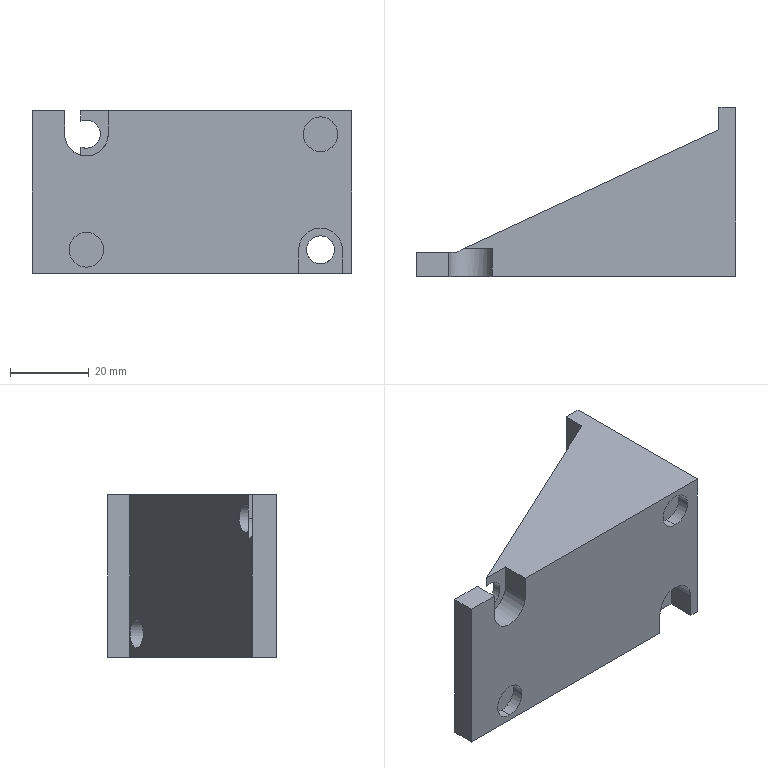Part | STEP file | 4-20.sldasm-Part-218 | 1 solid | 29 faces | box 81.175 x 42.9 x 41.3 mm | volume 66698 mm3 | plane 18 | cylinder 11 | commonest cylinder face diameters 7.142 x5 8.82 x4 11.112 x2
STEP:
#1=CARTESIAN_POINT('',(-270.795,-581.8,-57.11));
#2=VERTEX_POINT('',#1);
#3=CARTESIAN_POINT('',(-270.795,-581.8,-48.29));
#4=VERTEX_POINT('',#3);
#5=CARTESIAN_POINT('',(-270.795,-581.8,-52.7));
#6=DIRECTION('',(0.,1.,0.));
#7=DIRECTION('',(0.,0.,-1.));
#8=AXIS2_PLACEMENT_3D('',#5,#6,#7);
#9=CIRCLE('',#8,4.41);
#10=EDGE_CURVE('',#2,#4,#9,.T.);
#11=ORIENTED_EDGE('',*,*,#10,.F.);
#12=CARTESIAN_POINT('',(-270.795,-578.79,-57.11));
#13=VERTEX_POINT('',#12);
#14=CARTESIAN_POINT('',(-270.795,-583.99,-57.11));
#15=DIRECTION('',(0.,1.,0.));
#16=VECTOR('',#15,1000.);
#17=LINE('',#14,#16);
#18=EDGE_CURVE('',#2,#13,#17,.T.);
#19=ORIENTED_EDGE('',*,*,#18,.T.);
#20=CARTESIAN_POINT('',(-270.795,-578.79,-48.29));
#21=VERTEX_POINT('',#20);
#22=CARTESIAN_POINT('',(-270.795,-578.79,-52.7));
#23=DIRECTION('',(0.,-1.,0.));
#24=DIRECTION('',(0.,0.,-1.));
#25=AXIS2_PLACEMENT_3D('',#22,#23,#24);
#26=CIRCLE('',#25,4.41);
#27=EDGE_CURVE('',#21,#13,#26,.T.);
#28=ORIENTED_EDGE('',*,*,#27,.F.);
#29=CARTESIAN_POINT('',(-270.795,-583.99,-48.29));
#30=DIRECTION('',(0.,1.,0.));
#31=VECTOR('',#30,1000.);
#32=LINE('',#29,#31);
#33=EDGE_CURVE('',#4,#21,#32,.T.);
#34=ORIENTED_EDGE('',*,*,#33,.F.);
#35=EDGE_LOOP('',(#11,#19,#28,#34));
#36=FACE_OUTER_BOUND('',#35,.T.);
#37=CARTESIAN_POINT('',(-270.795,-583.99,-52.7));
#38=DIRECTION('',(0.,1.,0.));
#39=DIRECTION('',(0.,0.,1.));
#40=AXIS2_PLACEMENT_3D('',#37,#38,#39);
#41=CYLINDRICAL_SURFACE('',#40,4.41);
#42=ADVANCED_FACE('',(#36),#41,.F.);
#43=CARTESIAN_POINT('',(-211.295,-581.8,-18.89));
#44=VERTEX_POINT('',#43);
#45=CARTESIAN_POINT('',(-211.295,-581.8,-27.71));
#46=VERTEX_POINT('',#45);
#47=CARTESIAN_POINT('',(-211.295,-581.8,-23.3));
#48=DIRECTION('',(0.,-1.,0.));
#49=DIRECTION('',(0.,0.,-1.));
#50=AXIS2_PLACEMENT_3D('',#47,#48,#49);
#51=CIRCLE('',#50,4.41);
#52=EDGE_CURVE('',#44,#46,#51,.T.);
#53=ORIENTED_EDGE('',*,*,#52,.T.);
#54=CARTESIAN_POINT('',(-211.295,-578.678,-27.71));
#55=VERTEX_POINT('',#54);
#56=CARTESIAN_POINT('',(-211.295,-583.878,-27.71));
#57=DIRECTION('',(0.,1.,0.));
#58=VECTOR('',#57,1000.);
#59=LINE('',#56,#58);
#60=EDGE_CURVE('',#46,#55,#59,.T.);
#61=ORIENTED_EDGE('',*,*,#60,.T.);
#62=CARTESIAN_POINT('',(-211.295,-578.678,-18.89));
#63=VERTEX_POINT('',#62);
#64=CARTESIAN_POINT('',(-211.295,-578.678,-23.3));
#65=DIRECTION('',(0.,1.,0.));
#66=DIRECTION('',(0.,0.,1.));
#67=AXIS2_PLACEMENT_3D('',#64,#65,#66);
#68=CIRCLE('',#67,4.41);
#69=EDGE_CURVE('',#55,#63,#68,.T.);
#70=ORIENTED_EDGE('',*,*,#69,.T.);
#71=CARTESIAN_POINT('',(-211.295,-583.878,-18.89));
#72=DIRECTION('',(0.,1.,0.));
#73=VECTOR('',#72,1000.);
#74=LINE('',#71,#73);
#75=EDGE_CURVE('',#44,#63,#74,.T.);
#76=ORIENTED_EDGE('',*,*,#75,.F.);
#77=EDGE_LOOP('',(#53,#61,#70,#76));
#78=FACE_OUTER_BOUND('',#77,.T.);
#79=CARTESIAN_POINT('',(-211.295,-583.878,-23.3));
#80=DIRECTION('',(0.,1.,0.));
#81=DIRECTION('',(0.,0.,1.));
#82=AXIS2_PLACEMENT_3D('',#79,#80,#81);
#83=CYLINDRICAL_SURFACE('',#82,4.41);
#84=ADVANCED_FACE('',(#78),#83,.F.);
#85=CARTESIAN_POINT('',(-270.795,-574.688,-26.871));
#86=VERTEX_POINT('',#85);
#87=CARTESIAN_POINT('',(-270.795,-574.688,-19.729));
#88=VERTEX_POINT('',#87);
#89=CARTESIAN_POINT('',(-270.795,-574.688,-23.3));
#90=DIRECTION('',(0.,-1.,0.));
#91=DIRECTION('',(0.,0.,-1.));
#92=AXIS2_PLACEMENT_3D('',#89,#90,#91);
#93=CIRCLE('',#92,3.571);
#94=EDGE_CURVE('',#86,#88,#93,.T.);
#95=ORIENTED_EDGE('',*,*,#94,.T.);
#96=CARTESIAN_POINT('',(-270.795,-574.024,-19.729));
#97=VERTEX_POINT('',#96);
#98=CARTESIAN_POINT('',(-270.795,-574.688,-19.729));
#99=DIRECTION('',(0.,1.,0.));
#100=VECTOR('',#99,1000.);
#101=LINE('',#98,#100);
#102=EDGE_CURVE('',#88,#97,#101,.T.);
#103=ORIENTED_EDGE('',*,*,#102,.T.);
#104=CARTESIAN_POINT('',(-270.795,-574.024,-26.871));
#105=VERTEX_POINT('',#104);
#106=CARTESIAN_POINT('',(-270.795,-574.024,-26.871));
#107=CARTESIAN_POINT('',(-263.653,-570.694,-26.871));
#108=CARTESIAN_POINT('',(-263.653,-570.694,-19.729));
#109=CARTESIAN_POINT('',(-270.795,-574.024,-19.729));
#110=(BOUNDED_CURVE()B_SPLINE_CURVE(3,(#106,#107,#108,#109),.UNSPECIFIED.,.F.,.F.)B_SPLINE_CURVE_WITH_KNOTS((4,4),(4.712,7.854),.UNSPECIFIED.)CURVE()GEOMETRIC_REPRESENTATION_ITEM()RATIONAL_B_SPLINE_CURVE((1.,0.3333,0.3333,1.))REPRESENTATION_ITEM(''));
#111=EDGE_CURVE('',#105,#97,#110,.T.);
#112=ORIENTED_EDGE('',*,*,#111,.F.);
#113=CARTESIAN_POINT('',(-270.795,-574.688,-26.871));
#114=DIRECTION('',(0.,1.,0.));
#115=VECTOR('',#114,1000.);
#116=LINE('',#113,#115);
#117=EDGE_CURVE('',#86,#105,#116,.T.);
#118=ORIENTED_EDGE('',*,*,#117,.F.);
#119=EDGE_LOOP('',(#95,#103,#112,#118));
#120=FACE_OUTER_BOUND('',#119,.T.);
#121=CARTESIAN_POINT('',(-270.795,-574.688,-23.3));
#122=DIRECTION('',(0.,1.,0.));
#123=DIRECTION('',(0.,0.,-1.));
#124=AXIS2_PLACEMENT_3D('',#121,#122,#123);
#125=CYLINDRICAL_SURFACE('',#124,3.571);
#126=ADVANCED_FACE('',(#120),#125,.F.);
#127=CARTESIAN_POINT('',(-272.218,-574.688,-26.575));
#128=VERTEX_POINT('',#127);
#129=CARTESIAN_POINT('',(-270.795,-574.688,-23.3));
#130=DIRECTION('',(0.,-1.,0.));
#131=DIRECTION('',(0.,0.,-1.));
#132=AXIS2_PLACEMENT_3D('',#129,#130,#131);
#133=CIRCLE('',#132,3.571);
#134=EDGE_CURVE('',#128,#86,#133,.T.);
#135=ORIENTED_EDGE('',*,*,#134,.T.);
#136=ORIENTED_EDGE('',*,*,#117,.T.);
#137=CARTESIAN_POINT('',(-272.218,-574.688,-26.575));
#138=CARTESIAN_POINT('',(-271.767,-574.478,-26.771));
#139=CARTESIAN_POINT('',(-271.286,-574.254,-26.871));
#140=CARTESIAN_POINT('',(-270.795,-574.024,-26.871));
#141=(BOUNDED_CURVE()B_SPLINE_CURVE(3,(#137,#138,#139,#140),.UNSPECIFIED.,.F.,.T.)B_SPLINE_CURVE_WITH_KNOTS((4,4),(4.303,4.712),.UNSPECIFIED.)CURVE()GEOMETRIC_REPRESENTATION_ITEM()RATIONAL_B_SPLINE_CURVE((1.,0.986,0.986,1.))REPRESENTATION_ITEM(''));
#142=EDGE_CURVE('',#128,#105,#141,.T.);
#143=ORIENTED_EDGE('',*,*,#142,.F.);
#144=EDGE_LOOP('',(#135,#136,#143));
#145=FACE_OUTER_BOUND('',#144,.T.);
#146=CARTESIAN_POINT('',(-270.795,-574.688,-23.3));
#147=DIRECTION('',(0.,1.,0.));
#148=DIRECTION('',(0.,0.,-1.));
#149=AXIS2_PLACEMENT_3D('',#146,#147,#148);
#150=CYLINDRICAL_SURFACE('',#149,3.571);
#151=ADVANCED_FACE('',(#145),#150,.F.);
#152=CARTESIAN_POINT('',(-211.295,-574.688,-56.271));
#153=VERTEX_POINT('',#152);
#154=CARTESIAN_POINT('',(-211.295,-574.688,-49.129));
#155=VERTEX_POINT('',#154);
#156=CARTESIAN_POINT('',(-211.295,-574.688,-52.7));
#157=DIRECTION('',(0.,1.,0.));
#158=DIRECTION('',(0.,0.,1.));
#159=AXIS2_PLACEMENT_3D('',#156,#157,#158);
#160=CIRCLE('',#159,3.571);
#161=EDGE_CURVE('',#153,#155,#160,.T.);
#162=ORIENTED_EDGE('',*,*,#161,.F.);
#163=CARTESIAN_POINT('',(-211.295,-546.279,-56.271));
#164=VERTEX_POINT('',#163);
#165=CARTESIAN_POINT('',(-211.295,-574.688,-56.271));
#166=DIRECTION('',(0.,1.,0.));
#167=VECTOR('',#166,1000.);
#168=LINE('',#165,#167);
#169=EDGE_CURVE('',#153,#164,#168,.T.);
#170=ORIENTED_EDGE('',*,*,#169,.T.);
#171=CARTESIAN_POINT('',(-211.295,-546.279,-49.129));
#172=VERTEX_POINT('',#171);
#173=CARTESIAN_POINT('',(-211.295,-546.279,-49.129));
#174=CARTESIAN_POINT('',(-218.438,-549.61,-49.129));
#175=CARTESIAN_POINT('',(-218.438,-549.61,-56.271));
#176=CARTESIAN_POINT('',(-211.295,-546.279,-56.271));
#177=(BOUNDED_CURVE()B_SPLINE_CURVE(3,(#173,#174,#175,#176),.UNSPECIFIED.,.F.,.F.)B_SPLINE_CURVE_WITH_KNOTS((4,4),(1.571,4.712),.UNSPECIFIED.)CURVE()GEOMETRIC_REPRESENTATION_ITEM()RATIONAL_B_SPLINE_CURVE((1.,0.3333,0.3333,1.))REPRESENTATION_ITEM(''));
#178=EDGE_CURVE('',#172,#164,#177,.T.);
#179=ORIENTED_EDGE('',*,*,#178,.F.);
#180=CARTESIAN_POINT('',(-211.295,-574.688,-49.129));
#181=DIRECTION('',(0.,1.,0.));
#182=VECTOR('',#181,1000.);
#183=LINE('',#180,#182);
#184=EDGE_CURVE('',#155,#172,#183,.T.);
#185=ORIENTED_EDGE('',*,*,#184,.F.);
#186=EDGE_LOOP('',(#162,#170,#179,#185));
#187=FACE_OUTER_BOUND('',#186,.T.);
#188=CARTESIAN_POINT('',(-211.295,-574.688,-52.7));
#189=DIRECTION('',(0.,1.,0.));
#190=DIRECTION('',(0.,0.,1.));
#191=AXIS2_PLACEMENT_3D('',#188,#189,#190);
#192=CYLINDRICAL_SURFACE('',#191,3.571);
#193=ADVANCED_FACE('',(#187),#192,.F.);
#194=ORIENTED_EDGE('',*,*,#52,.F.);
#195=CARTESIAN_POINT('',(-211.295,-581.8,-23.3));
#196=DIRECTION('',(0.,-1.,0.));
#197=DIRECTION('',(0.,0.,-1.));
#198=AXIS2_PLACEMENT_3D('',#195,#196,#197);
#199=CIRCLE('',#198,4.41);
#200=EDGE_CURVE('',#46,#44,#199,.T.);
#201=ORIENTED_EDGE('',*,*,#200,.F.);
#202=EDGE_LOOP('',(#194,#201));
#203=FACE_BOUND('',#202,.T.);
#204=CARTESIAN_POINT('',(-270.795,-581.8,-52.7));
#205=DIRECTION('',(0.,1.,0.));
#206=DIRECTION('',(0.,0.,-1.));
#207=AXIS2_PLACEMENT_3D('',#204,#205,#206);
#208=CIRCLE('',#207,4.41);
#209=EDGE_CURVE('',#4,#2,#208,.T.);
#210=ORIENTED_EDGE('',*,*,#209,.T.);
#211=ORIENTED_EDGE('',*,*,#10,.T.);
#212=EDGE_LOOP('',(#210,#211));
#213=FACE_BOUND('',#212,.T.);
#214=CARTESIAN_POINT('',(-216.851,-581.8,-58.65));
#215=VERTEX_POINT('',#214);
#216=CARTESIAN_POINT('',(-284.545,-581.8,-58.65));
#217=VERTEX_POINT('',#216);
#218=CARTESIAN_POINT('',(-232.845,-581.8,-58.65));
#219=DIRECTION('',(-1.,0.,0.));
#220=VECTOR('',#219,1000.);
#221=LINE('',#218,#220);
#222=EDGE_CURVE('',#215,#217,#221,.T.);
#223=ORIENTED_EDGE('',*,*,#222,.F.);
#224=CARTESIAN_POINT('',(-216.851,-581.8,-52.7));
#225=VERTEX_POINT('',#224);
#226=CARTESIAN_POINT('',(-216.851,-581.8,-64.256));
#227=DIRECTION('',(0.,0.,1.));
#228=VECTOR('',#227,1000.);
#229=LINE('',#226,#228);
#230=EDGE_CURVE('',#215,#225,#229,.T.);
#231=ORIENTED_EDGE('',*,*,#230,.T.);
#232=CARTESIAN_POINT('',(-205.739,-581.8,-52.7));
#233=VERTEX_POINT('',#232);
#234=CARTESIAN_POINT('',(-211.295,-581.8,-52.7));
#235=DIRECTION('',(0.,-1.,0.));
#236=DIRECTION('',(0.,0.,-1.));
#237=AXIS2_PLACEMENT_3D('',#234,#235,#236);
#238=CIRCLE('',#237,5.556);
#239=EDGE_CURVE('',#233,#225,#238,.T.);
#240=ORIENTED_EDGE('',*,*,#239,.F.);
#241=CARTESIAN_POINT('',(-205.739,-581.8,-58.65));
#242=VERTEX_POINT('',#241);
#243=CARTESIAN_POINT('',(-205.739,-581.8,-64.256));
#244=DIRECTION('',(0.,0.,1.));
#245=VECTOR('',#244,1000.);
#246=LINE('',#243,#245);
#247=EDGE_CURVE('',#242,#233,#246,.T.);
#248=ORIENTED_EDGE('',*,*,#247,.F.);
#249=CARTESIAN_POINT('',(-203.37,-581.8,-58.65));
#250=VERTEX_POINT('',#249);
#251=CARTESIAN_POINT('',(-232.845,-581.8,-58.65));
#252=DIRECTION('',(-1.,0.,0.));
#253=VECTOR('',#252,1000.);
#254=LINE('',#251,#253);
#255=EDGE_CURVE('',#250,#242,#254,.T.);
#256=ORIENTED_EDGE('',*,*,#255,.F.);
#257=CARTESIAN_POINT('',(-203.37,-581.8,-17.35));
#258=VERTEX_POINT('',#257);
#259=CARTESIAN_POINT('',(-203.37,-581.8,-38.));
#260=DIRECTION('',(0.,0.,1.));
#261=VECTOR('',#260,1000.);
#262=LINE('',#259,#261);
#263=EDGE_CURVE('',#250,#258,#262,.T.);
#264=ORIENTED_EDGE('',*,*,#263,.T.);
#265=CARTESIAN_POINT('',(-265.239,-581.8,-17.35));
#266=VERTEX_POINT('',#265);
#267=CARTESIAN_POINT('',(-232.845,-581.8,-17.35));
#268=DIRECTION('',(1.,0.,0.));
#269=VECTOR('',#268,1000.);
#270=LINE('',#267,#269);
#271=EDGE_CURVE('',#266,#258,#270,.T.);
#272=ORIENTED_EDGE('',*,*,#271,.F.);
#273=CARTESIAN_POINT('',(-265.239,-581.8,-23.3));
#274=VERTEX_POINT('',#273);
#275=CARTESIAN_POINT('',(-265.239,-581.8,-28.856));
#276=DIRECTION('',(0.,0.,1.));
#277=VECTOR('',#276,1000.);
#278=LINE('',#275,#277);
#279=EDGE_CURVE('',#274,#266,#278,.T.);
#280=ORIENTED_EDGE('',*,*,#279,.F.);
#281=CARTESIAN_POINT('',(-276.351,-581.8,-23.3));
#282=VERTEX_POINT('',#281);
#283=CARTESIAN_POINT('',(-270.795,-581.8,-23.3));
#284=DIRECTION('',(0.,1.,0.));
#285=DIRECTION('',(0.,0.,1.));
#286=AXIS2_PLACEMENT_3D('',#283,#284,#285);
#287=CIRCLE('',#286,5.556);
#288=EDGE_CURVE('',#274,#282,#287,.T.);
#289=ORIENTED_EDGE('',*,*,#288,.T.);
#290=CARTESIAN_POINT('',(-276.351,-581.8,-17.35));
#291=VERTEX_POINT('',#290);
#292=CARTESIAN_POINT('',(-276.351,-581.8,-28.856));
#293=DIRECTION('',(0.,0.,1.));
#294=VECTOR('',#293,1000.);
#295=LINE('',#292,#294);
#296=EDGE_CURVE('',#282,#291,#295,.T.);
#297=ORIENTED_EDGE('',*,*,#296,.T.);
#298=CARTESIAN_POINT('',(-284.545,-581.8,-17.35));
#299=VERTEX_POINT('',#298);
#300=CARTESIAN_POINT('',(-232.845,-581.8,-17.35));
#301=DIRECTION('',(1.,0.,0.));
#302=VECTOR('',#301,1000.);
#303=LINE('',#300,#302);
#304=EDGE_CURVE('',#299,#291,#303,.T.);
#305=ORIENTED_EDGE('',*,*,#304,.F.);
#306=CARTESIAN_POINT('',(-284.545,-581.8,-38.));
#307=DIRECTION('',(0.,0.,1.));
#308=VECTOR('',#307,1000.);
#309=LINE('',#306,#308);
#310=EDGE_CURVE('',#217,#299,#309,.T.);
#311=ORIENTED_EDGE('',*,*,#310,.F.);
#312=EDGE_LOOP('',(#223,#231,#240,#248,#256,#264,#272,#280,#289,#297,#305,#311));
#313=FACE_OUTER_BOUND('',#312,.T.);
#314=CARTESIAN_POINT('',(-232.845,-581.8,-38.));
#315=DIRECTION('',(0.,-1.,0.));
#316=DIRECTION('',(0.,0.,-1.));
#317=AXIS2_PLACEMENT_3D('',#314,#315,#316);
#318=PLANE('',#317);
#319=ADVANCED_FACE('',(#203,#213,#313),#318,.T.);
#320=CARTESIAN_POINT('',(-276.351,-575.7,-17.35));
#321=VERTEX_POINT('',#320);
#322=CARTESIAN_POINT('',(-276.351,-535.,-17.35));
#323=DIRECTION('',(0.,-1.,0.));
#324=VECTOR('',#323,1000.);
#325=LINE('',#322,#324);
#326=EDGE_CURVE('',#321,#291,#325,.T.);
#327=ORIENTED_EDGE('',*,*,#326,.F.);
#328=CARTESIAN_POINT('',(-284.545,-575.7,-17.35));
#329=VERTEX_POINT('',#328);
#330=CARTESIAN_POINT('',(-246.645,-575.7,-17.35));
#331=DIRECTION('',(-1.,0.,0.));
#332=VECTOR('',#331,1000.);
#333=LINE('',#330,#332);
#334=EDGE_CURVE('',#321,#329,#333,.T.);
#335=ORIENTED_EDGE('',*,*,#334,.T.);
#336=CARTESIAN_POINT('',(-284.545,-535.,-17.35));
#337=DIRECTION('',(0.,-1.,0.));
#338=VECTOR('',#337,1000.);
#339=LINE('',#336,#338);
#340=EDGE_CURVE('',#329,#299,#339,.T.);
#341=ORIENTED_EDGE('',*,*,#340,.T.);
#342=ORIENTED_EDGE('',*,*,#304,.T.);
#343=EDGE_LOOP('',(#327,#335,#341,#342));
#344=FACE_OUTER_BOUND('',#343,.T.);
#345=CARTESIAN_POINT('',(-232.845,-535.,-17.35));
#346=DIRECTION('',(0.,0.,1.));
#347=DIRECTION('',(0.,-1.,0.));
#348=AXIS2_PLACEMENT_3D('',#345,#346,#347);
#349=PLANE('',#348);
#350=ADVANCED_FACE('',(#344),#349,.T.);
#351=CARTESIAN_POINT('',(-276.351,-575.7,-23.3));
#352=VERTEX_POINT('',#351);
#353=CARTESIAN_POINT('',(-276.351,-578.244,-23.3));
#354=DIRECTION('',(0.,-1.,0.));
#355=VECTOR('',#354,1000.);
#356=LINE('',#353,#355);
#357=EDGE_CURVE('',#352,#282,#356,.T.);
#358=ORIENTED_EDGE('',*,*,#357,.T.);
#359=ORIENTED_EDGE('',*,*,#288,.F.);
#360=CARTESIAN_POINT('',(-265.239,-574.688,-23.3));
#361=VERTEX_POINT('',#360);
#362=CARTESIAN_POINT('',(-265.239,-578.244,-23.3));
#363=DIRECTION('',(0.,1.,0.));
#364=VECTOR('',#363,1000.);
#365=LINE('',#362,#364);
#366=EDGE_CURVE('',#274,#361,#365,.T.);
#367=ORIENTED_EDGE('',*,*,#366,.T.);
#368=CARTESIAN_POINT('',(-272.218,-574.688,-28.671));
#369=VERTEX_POINT('',#368);
#370=CARTESIAN_POINT('',(-270.795,-574.688,-23.3));
#371=DIRECTION('',(0.,1.,0.));
#372=DIRECTION('',(0.,0.,1.));
#373=AXIS2_PLACEMENT_3D('',#370,#371,#372);
#374=CIRCLE('',#373,5.556);
#375=EDGE_CURVE('',#361,#369,#374,.T.);
#376=ORIENTED_EDGE('',*,*,#375,.T.);
#377=CARTESIAN_POINT('',(-274.388,-575.7,-27.538));
#378=VERTEX_POINT('',#377);
#379=CARTESIAN_POINT('',(-274.388,-575.7,-27.538));
#380=CARTESIAN_POINT('',(-273.756,-575.405,-28.074));
#381=CARTESIAN_POINT('',(-273.02,-575.062,-28.458));
#382=CARTESIAN_POINT('',(-272.218,-574.688,-28.671));
#383=(BOUNDED_CURVE()B_SPLINE_CURVE(3,(#379,#380,#381,#382),.UNSPECIFIED.,.F.,.F.)B_SPLINE_CURVE_WITH_KNOTS((4,4),(0.8675,1.312),.UNSPECIFIED.)CURVE()GEOMETRIC_REPRESENTATION_ITEM()RATIONAL_B_SPLINE_CURVE((1.,0.9836,0.9836,1.))REPRESENTATION_ITEM(''));
#384=EDGE_CURVE('',#378,#369,#383,.T.);
#385=ORIENTED_EDGE('',*,*,#384,.F.);
#386=CARTESIAN_POINT('',(-270.795,-575.7,-23.3));
#387=DIRECTION('',(0.,-1.,0.));
#388=DIRECTION('',(0.,0.,-1.));
#389=AXIS2_PLACEMENT_3D('',#386,#387,#388);
#390=CIRCLE('',#389,5.556);
#391=EDGE_CURVE('',#352,#378,#390,.T.);
#392=ORIENTED_EDGE('',*,*,#391,.F.);
#393=EDGE_LOOP('',(#358,#359,#367,#376,#385,#392));
#394=FACE_OUTER_BOUND('',#393,.T.);
#395=CARTESIAN_POINT('',(-270.795,-574.688,-23.3));
#396=DIRECTION('',(0.,-1.,0.));
#397=DIRECTION('',(0.,0.,1.));
#398=AXIS2_PLACEMENT_3D('',#395,#396,#397);
#399=CYLINDRICAL_SURFACE('',#398,5.556);
#400=ADVANCED_FACE('',(#394),#399,.F.);
#401=CARTESIAN_POINT('',(-216.851,-574.688,-58.65));
#402=VERTEX_POINT('',#401);
#403=CARTESIAN_POINT('',(-216.851,-535.,-58.65));
#404=DIRECTION('',(0.,1.,0.));
#405=VECTOR('',#404,1000.);
#406=LINE('',#403,#405);
#407=EDGE_CURVE('',#215,#402,#406,.T.);
#408=ORIENTED_EDGE('',*,*,#407,.F.);
#409=ORIENTED_EDGE('',*,*,#222,.T.);
#410=CARTESIAN_POINT('',(-284.545,-575.7,-58.65));
#411=VERTEX_POINT('',#410);
#412=CARTESIAN_POINT('',(-284.545,-535.,-58.65));
#413=DIRECTION('',(0.,-1.,0.));
#414=VECTOR('',#413,1000.);
#415=LINE('',#412,#414);
#416=EDGE_CURVE('',#411,#217,#415,.T.);
#417=ORIENTED_EDGE('',*,*,#416,.F.);
#418=CARTESIAN_POINT('',(-274.388,-575.7,-58.65));
#419=VERTEX_POINT('',#418);
#420=CARTESIAN_POINT('',(-246.645,-575.7,-58.65));
#421=DIRECTION('',(1.,0.,0.));
#422=VECTOR('',#421,1000.);
#423=LINE('',#420,#422);
#424=EDGE_CURVE('',#411,#419,#423,.T.);
#425=ORIENTED_EDGE('',*,*,#424,.T.);
#426=CARTESIAN_POINT('',(-207.645,-544.577,-58.65));
#427=VERTEX_POINT('',#426);
#428=CARTESIAN_POINT('',(-243.748,-561.412,-58.65));
#429=DIRECTION('',(-0.9063,-0.4226,0.));
#430=VECTOR('',#429,1000.);
#431=LINE('',#428,#430);
#432=EDGE_CURVE('',#427,#419,#431,.T.);
#433=ORIENTED_EDGE('',*,*,#432,.F.);
#434=CARTESIAN_POINT('',(-207.645,-538.9,-58.65));
#435=VERTEX_POINT('',#434);
#436=CARTESIAN_POINT('',(-207.645,-555.2,-58.65));
#437=DIRECTION('',(0.,1.,0.));
#438=VECTOR('',#437,1000.);
#439=LINE('',#436,#438);
#440=EDGE_CURVE('',#427,#435,#439,.T.);
#441=ORIENTED_EDGE('',*,*,#440,.T.);
#442=CARTESIAN_POINT('',(-203.37,-538.9,-58.65));
#443=VERTEX_POINT('',#442);
#444=CARTESIAN_POINT('',(-232.845,-538.9,-58.65));
#445=DIRECTION('',(1.,0.,0.));
#446=VECTOR('',#445,1000.);
#447=LINE('',#444,#446);
#448=EDGE_CURVE('',#435,#443,#447,.T.);
#449=ORIENTED_EDGE('',*,*,#448,.T.);
#450=CARTESIAN_POINT('',(-203.37,-535.,-58.65));
#451=DIRECTION('',(0.,-1.,0.));
#452=VECTOR('',#451,1000.);
#453=LINE('',#450,#452);
#454=EDGE_CURVE('',#443,#250,#453,.T.);
#455=ORIENTED_EDGE('',*,*,#454,.T.);
#456=ORIENTED_EDGE('',*,*,#255,.T.);
#457=CARTESIAN_POINT('',(-205.739,-574.688,-58.65));
#458=VERTEX_POINT('',#457);
#459=CARTESIAN_POINT('',(-205.739,-535.,-58.65));
#460=DIRECTION('',(0.,-1.,0.));
#461=VECTOR('',#460,1000.);
#462=LINE('',#459,#461);
#463=EDGE_CURVE('',#458,#242,#462,.T.);
#464=ORIENTED_EDGE('',*,*,#463,.F.);
#465=CARTESIAN_POINT('',(-232.845,-574.688,-58.65));
#466=DIRECTION('',(1.,0.,0.));
#467=VECTOR('',#466,1000.);
#468=LINE('',#465,#467);
#469=EDGE_CURVE('',#402,#458,#468,.T.);
#470=ORIENTED_EDGE('',*,*,#469,.F.);
#471=EDGE_LOOP('',(#408,#409,#417,#425,#433,#441,#449,#455,#456,#464,#470));
#472=FACE_OUTER_BOUND('',#471,.T.);
#473=CARTESIAN_POINT('',(-232.845,-535.,-58.65));
#474=DIRECTION('',(0.,0.,-1.));
#475=DIRECTION('',(0.,1.,0.));
#476=AXIS2_PLACEMENT_3D('',#473,#474,#475);
#477=PLANE('',#476);
#478=ADVANCED_FACE('',(#472),#477,.T.);
#479=CARTESIAN_POINT('',(-265.239,-574.688,-17.35));
#480=VERTEX_POINT('',#479);
#481=CARTESIAN_POINT('',(-272.218,-574.688,-17.35));
#482=VERTEX_POINT('',#481);
#483=CARTESIAN_POINT('',(-232.845,-574.688,-17.35));
#484=DIRECTION('',(-1.,0.,0.));
#485=VECTOR('',#484,1000.);
#486=LINE('',#483,#485);
#487=EDGE_CURVE('',#480,#482,#486,.T.);
#488=ORIENTED_EDGE('',*,*,#487,.F.);
#489=CARTESIAN_POINT('',(-265.239,-535.,-17.35));
#490=DIRECTION('',(0.,1.,0.));
#491=VECTOR('',#490,1000.);
#492=LINE('',#489,#491);
#493=EDGE_CURVE('',#266,#480,#492,.T.);
#494=ORIENTED_EDGE('',*,*,#493,.F.);
#495=ORIENTED_EDGE('',*,*,#271,.T.);
#496=CARTESIAN_POINT('',(-203.37,-538.9,-17.35));
#497=VERTEX_POINT('',#496);
#498=CARTESIAN_POINT('',(-203.37,-535.,-17.35));
#499=DIRECTION('',(0.,1.,0.));
#500=VECTOR('',#499,1000.);
#501=LINE('',#498,#500);
#502=EDGE_CURVE('',#258,#497,#501,.T.);
#503=ORIENTED_EDGE('',*,*,#502,.T.);
#504=CARTESIAN_POINT('',(-207.645,-538.9,-17.35));
#505=VERTEX_POINT('',#504);
#506=CARTESIAN_POINT('',(-232.845,-538.9,-17.35));
#507=DIRECTION('',(-1.,0.,0.));
#508=VECTOR('',#507,1000.);
#509=LINE('',#506,#508);
#510=EDGE_CURVE('',#497,#505,#509,.T.);
#511=ORIENTED_EDGE('',*,*,#510,.T.);
#512=CARTESIAN_POINT('',(-207.645,-544.577,-17.35));
#513=VERTEX_POINT('',#512);
#514=CARTESIAN_POINT('',(-207.645,-555.2,-17.35));
#515=DIRECTION('',(0.,-1.,0.));
#516=VECTOR('',#515,1000.);
#517=LINE('',#514,#516);
#518=EDGE_CURVE('',#505,#513,#517,.T.);
#519=ORIENTED_EDGE('',*,*,#518,.T.);
#520=CARTESIAN_POINT('',(-243.748,-561.412,-17.35));
#521=DIRECTION('',(0.9063,0.4226,0.));
#522=VECTOR('',#521,1000.);
#523=LINE('',#520,#522);
#524=EDGE_CURVE('',#482,#513,#523,.T.);
#525=ORIENTED_EDGE('',*,*,#524,.F.);
#526=EDGE_LOOP('',(#488,#494,#495,#503,#511,#519,#525));
#527=FACE_OUTER_BOUND('',#526,.T.);
#528=CARTESIAN_POINT('',(-232.845,-535.,-17.35));
#529=DIRECTION('',(0.,0.,1.));
#530=DIRECTION('',(0.,-1.,0.));
#531=AXIS2_PLACEMENT_3D('',#528,#529,#530);
#532=PLANE('',#531);
#533=ADVANCED_FACE('',(#527),#532,.T.);
#534=CARTESIAN_POINT('',(-207.645,-538.9,-38.));
#535=DIRECTION('',(0.,0.,-1.));
#536=VECTOR('',#535,1000.);
#537=LINE('',#534,#536);
#538=EDGE_CURVE('',#505,#435,#537,.T.);
#539=ORIENTED_EDGE('',*,*,#538,.F.);
#540=ORIENTED_EDGE('',*,*,#510,.F.);
#541=CARTESIAN_POINT('',(-203.37,-538.9,-38.));
#542=DIRECTION('',(0.,0.,-1.));
#543=VECTOR('',#542,1000.);
#544=LINE('',#541,#543);
#545=EDGE_CURVE('',#497,#443,#544,.T.);
#546=ORIENTED_EDGE('',*,*,#545,.T.);
#547=ORIENTED_EDGE('',*,*,#448,.F.);
#548=EDGE_LOOP('',(#539,#540,#546,#547));
#549=FACE_OUTER_BOUND('',#548,.T.);
#550=CARTESIAN_POINT('',(-232.845,-538.9,-38.));
#551=DIRECTION('',(0.,1.,0.));
#552=DIRECTION('',(0.,0.,1.));
#553=AXIS2_PLACEMENT_3D('',#550,#551,#552);
#554=PLANE('',#553);
#555=ADVANCED_FACE('',(#549),#554,.T.);
#556=ORIENTED_EDGE('',*,*,#263,.F.);
#557=ORIENTED_EDGE('',*,*,#454,.F.);
#558=ORIENTED_EDGE('',*,*,#545,.F.);
#559=ORIENTED_EDGE('',*,*,#502,.F.);
#560=EDGE_LOOP('',(#556,#557,#558,#559));
#561=FACE_OUTER_BOUND('',#560,.T.);
#562=CARTESIAN_POINT('',(-203.37,-558.4,-38.));
#563=DIRECTION('',(1.,0.,0.));
#564=DIRECTION('',(0.,-1.,0.));
#565=AXIS2_PLACEMENT_3D('',#562,#563,#564);
#566=PLANE('',#565);
#567=ADVANCED_FACE('',(#561),#566,.T.);
#568=CARTESIAN_POINT('',(-284.545,-575.7,-38.));
#569=DIRECTION('',(0.,0.,1.));
#570=VECTOR('',#569,1000.);
#571=LINE('',#568,#570);
#572=EDGE_CURVE('',#411,#329,#571,.T.);
#573=ORIENTED_EDGE('',*,*,#572,.F.);
#574=ORIENTED_EDGE('',*,*,#416,.T.);
#575=ORIENTED_EDGE('',*,*,#310,.T.);
#576=ORIENTED_EDGE('',*,*,#340,.F.);
#577=EDGE_LOOP('',(#573,#574,#575,#576));
#578=FACE_OUTER_BOUND('',#577,.T.);
#579=CARTESIAN_POINT('',(-284.545,-535.,-38.));
#580=DIRECTION('',(-1.,0.,0.));
#581=DIRECTION('',(0.,1.,0.));
#582=AXIS2_PLACEMENT_3D('',#579,#580,#581);
#583=PLANE('',#582);
#584=ADVANCED_FACE('',(#578),#583,.T.);
#585=ORIENTED_EDGE('',*,*,#334,.F.);
#586=CARTESIAN_POINT('',(-276.351,-575.7,-58.65));
#587=DIRECTION('',(0.,0.,-1.));
#588=VECTOR('',#587,1000.);
#589=LINE('',#586,#588);
#590=EDGE_CURVE('',#321,#352,#589,.T.);
#591=ORIENTED_EDGE('',*,*,#590,.T.);
#592=ORIENTED_EDGE('',*,*,#391,.T.);
#593=CARTESIAN_POINT('',(-274.388,-575.7,-58.65));
#594=DIRECTION('',(0.,0.,1.));
#595=VECTOR('',#594,1000.);
#596=LINE('',#593,#595);
#597=EDGE_CURVE('',#419,#378,#596,.T.);
#598=ORIENTED_EDGE('',*,*,#597,.F.);
#599=ORIENTED_EDGE('',*,*,#424,.F.);
#600=ORIENTED_EDGE('',*,*,#572,.T.);
#601=EDGE_LOOP('',(#585,#591,#592,#598,#599,#600));
#602=FACE_OUTER_BOUND('',#601,.T.);
#603=CARTESIAN_POINT('',(-246.645,-575.7,-58.65));
#604=DIRECTION('',(0.,-1.,0.));
#605=DIRECTION('',(0.,0.,-1.));
#606=AXIS2_PLACEMENT_3D('',#603,#604,#605);
#607=PLANE('',#606);
#608=ADVANCED_FACE('',(#602),#607,.F.);
#609=CARTESIAN_POINT('',(-272.218,-574.688,-20.025));
#610=VERTEX_POINT('',#609);
#611=CARTESIAN_POINT('',(-272.218,-574.688,-58.65));
#612=DIRECTION('',(0.,0.,1.));
#613=VECTOR('',#612,1000.);
#614=LINE('',#611,#613);
#615=EDGE_CURVE('',#610,#482,#614,.T.);
#616=ORIENTED_EDGE('',*,*,#615,.T.);
#617=ORIENTED_EDGE('',*,*,#524,.T.);
#618=CARTESIAN_POINT('',(-207.645,-544.577,-58.65));
#619=DIRECTION('',(0.,0.,-1.));
#620=VECTOR('',#619,1000.);
#621=LINE('',#618,#620);
#622=EDGE_CURVE('',#513,#427,#621,.T.);
#623=ORIENTED_EDGE('',*,*,#622,.T.);
#624=ORIENTED_EDGE('',*,*,#432,.T.);
#625=ORIENTED_EDGE('',*,*,#597,.T.);
#626=ORIENTED_EDGE('',*,*,#384,.T.);
#627=CARTESIAN_POINT('',(-272.218,-574.688,-58.65));
#628=DIRECTION('',(0.,0.,1.));
#629=VECTOR('',#628,1000.);
#630=LINE('',#627,#629);
#631=EDGE_CURVE('',#369,#128,#630,.T.);
#632=ORIENTED_EDGE('',*,*,#631,.T.);
#633=ORIENTED_EDGE('',*,*,#142,.T.);
#634=ORIENTED_EDGE('',*,*,#111,.T.);
#635=CARTESIAN_POINT('',(-270.795,-574.024,-19.729));
#636=CARTESIAN_POINT('',(-271.286,-574.254,-19.729));
#637=CARTESIAN_POINT('',(-271.767,-574.478,-19.829));
#638=CARTESIAN_POINT('',(-272.218,-574.688,-20.025));
#639=(BOUNDED_CURVE()B_SPLINE_CURVE(3,(#635,#636,#637,#638),.UNSPECIFIED.,.F.,.F.)B_SPLINE_CURVE_WITH_KNOTS((4,4),(1.571,1.981),.UNSPECIFIED.)CURVE()GEOMETRIC_REPRESENTATION_ITEM()RATIONAL_B_SPLINE_CURVE((1.,0.986,0.986,1.))REPRESENTATION_ITEM(''));
#640=EDGE_CURVE('',#97,#610,#639,.T.);
#641=ORIENTED_EDGE('',*,*,#640,.T.);
#642=EDGE_LOOP('',(#616,#617,#623,#624,#625,#626,#632,#633,#634,#641));
#643=FACE_OUTER_BOUND('',#642,.T.);
#644=ORIENTED_EDGE('',*,*,#178,.T.);
#645=CARTESIAN_POINT('',(-211.295,-546.279,-56.271));
#646=CARTESIAN_POINT('',(-204.153,-542.948,-56.271));
#647=CARTESIAN_POINT('',(-204.153,-542.948,-49.129));
#648=CARTESIAN_POINT('',(-211.295,-546.279,-49.129));
#649=(BOUNDED_CURVE()B_SPLINE_CURVE(3,(#645,#646,#647,#648),.UNSPECIFIED.,.F.,.F.)B_SPLINE_CURVE_WITH_KNOTS((4,4),(4.712,7.854),.UNSPECIFIED.)CURVE()GEOMETRIC_REPRESENTATION_ITEM()RATIONAL_B_SPLINE_CURVE((1.,0.3333,0.3333,1.))REPRESENTATION_ITEM(''));
#650=EDGE_CURVE('',#164,#172,#649,.T.);
#651=ORIENTED_EDGE('',*,*,#650,.T.);
#652=EDGE_LOOP('',(#644,#651));
#653=FACE_BOUND('',#652,.T.);
#654=CARTESIAN_POINT('',(-273.745,-575.4,-58.65));
#655=DIRECTION('',(-0.4226,0.9063,0.));
#656=DIRECTION('',(-0.9063,-0.4226,0.));
#657=AXIS2_PLACEMENT_3D('',#654,#655,#656);
#658=PLANE('',#657);
#659=ADVANCED_FACE('',(#643,#653),#658,.T.);
#660=ORIENTED_EDGE('',*,*,#538,.T.);
#661=ORIENTED_EDGE('',*,*,#440,.F.);
#662=ORIENTED_EDGE('',*,*,#622,.F.);
#663=ORIENTED_EDGE('',*,*,#518,.F.);
#664=EDGE_LOOP('',(#660,#661,#662,#663));
#665=FACE_OUTER_BOUND('',#664,.T.);
#666=CARTESIAN_POINT('',(-207.645,-555.2,-58.65));
#667=DIRECTION('',(1.,0.,0.));
#668=DIRECTION('',(0.,0.,1.));
#669=AXIS2_PLACEMENT_3D('',#666,#667,#668);
#670=PLANE('',#669);
#671=ADVANCED_FACE('',(#665),#670,.F.);
#672=ORIENTED_EDGE('',*,*,#169,.F.);
#673=CARTESIAN_POINT('',(-211.295,-574.688,-52.7));
#674=DIRECTION('',(0.,1.,0.));
#675=DIRECTION('',(0.,0.,1.));
#676=AXIS2_PLACEMENT_3D('',#673,#674,#675);
#677=CIRCLE('',#676,3.571);
#678=EDGE_CURVE('',#155,#153,#677,.T.);
#679=ORIENTED_EDGE('',*,*,#678,.F.);
#680=ORIENTED_EDGE('',*,*,#184,.T.);
#681=ORIENTED_EDGE('',*,*,#650,.F.);
#682=EDGE_LOOP('',(#672,#679,#680,#681));
#683=FACE_OUTER_BOUND('',#682,.T.);
#684=CARTESIAN_POINT('',(-211.295,-574.688,-52.7));
#685=DIRECTION('',(0.,1.,0.));
#686=DIRECTION('',(0.,0.,1.));
#687=AXIS2_PLACEMENT_3D('',#684,#685,#686);
#688=CYLINDRICAL_SURFACE('',#687,3.571);
#689=ADVANCED_FACE('',(#683),#688,.F.);
#690=ORIENTED_EDGE('',*,*,#239,.T.);
#691=CARTESIAN_POINT('',(-216.851,-574.688,-52.7));
#692=VERTEX_POINT('',#691);
#693=CARTESIAN_POINT('',(-216.851,-578.244,-52.7));
#694=DIRECTION('',(0.,1.,0.));
#695=VECTOR('',#694,1000.);
#696=LINE('',#693,#695);
#697=EDGE_CURVE('',#225,#692,#696,.T.);
#698=ORIENTED_EDGE('',*,*,#697,.T.);
#699=CARTESIAN_POINT('',(-205.739,-574.688,-52.7));
#700=VERTEX_POINT('',#699);
#701=CARTESIAN_POINT('',(-211.295,-574.688,-52.7));
#702=DIRECTION('',(0.,-1.,0.));
#703=DIRECTION('',(0.,0.,-1.));
#704=AXIS2_PLACEMENT_3D('',#701,#702,#703);
#705=CIRCLE('',#704,5.556);
#706=EDGE_CURVE('',#700,#692,#705,.T.);
#707=ORIENTED_EDGE('',*,*,#706,.F.);
#708=CARTESIAN_POINT('',(-205.739,-578.244,-52.7));
#709=DIRECTION('',(0.,-1.,0.));
#710=VECTOR('',#709,1000.);
#711=LINE('',#708,#710);
#712=EDGE_CURVE('',#700,#233,#711,.T.);
#713=ORIENTED_EDGE('',*,*,#712,.T.);
#714=EDGE_LOOP('',(#690,#698,#707,#713));
#715=FACE_OUTER_BOUND('',#714,.T.);
#716=CARTESIAN_POINT('',(-211.295,-574.688,-52.7));
#717=DIRECTION('',(0.,-1.,0.));
#718=DIRECTION('',(0.,0.,-1.));
#719=AXIS2_PLACEMENT_3D('',#716,#717,#718);
#720=CYLINDRICAL_SURFACE('',#719,5.556);
#721=ADVANCED_FACE('',(#715),#720,.F.);
#722=ORIENTED_EDGE('',*,*,#678,.T.);
#723=ORIENTED_EDGE('',*,*,#161,.T.);
#724=EDGE_LOOP('',(#722,#723));
#725=FACE_BOUND('',#724,.T.);
#726=ORIENTED_EDGE('',*,*,#706,.T.);
#727=CARTESIAN_POINT('',(-216.851,-574.688,-64.256));
#728=DIRECTION('',(0.,0.,1.));
#729=VECTOR('',#728,1000.);
#730=LINE('',#727,#729);
#731=EDGE_CURVE('',#402,#692,#730,.T.);
#732=ORIENTED_EDGE('',*,*,#731,.F.);
#733=ORIENTED_EDGE('',*,*,#469,.T.);
#734=CARTESIAN_POINT('',(-205.739,-574.688,-64.256));
#735=DIRECTION('',(0.,0.,1.));
#736=VECTOR('',#735,1000.);
#737=LINE('',#734,#736);
#738=EDGE_CURVE('',#458,#700,#737,.T.);
#739=ORIENTED_EDGE('',*,*,#738,.T.);
#740=EDGE_LOOP('',(#726,#732,#733,#739));
#741=FACE_OUTER_BOUND('',#740,.T.);
#742=CARTESIAN_POINT('',(-211.295,-574.688,-52.7));
#743=DIRECTION('',(0.,1.,0.));
#744=DIRECTION('',(0.,0.,1.));
#745=AXIS2_PLACEMENT_3D('',#742,#743,#744);
#746=PLANE('',#745);
#747=ADVANCED_FACE('',(#725,#741),#746,.F.);
#748=ORIENTED_EDGE('',*,*,#487,.T.);
#749=ORIENTED_EDGE('',*,*,#615,.F.);
#750=CARTESIAN_POINT('',(-270.795,-574.688,-23.3));
#751=DIRECTION('',(0.,-1.,0.));
#752=DIRECTION('',(0.,0.,-1.));
#753=AXIS2_PLACEMENT_3D('',#750,#751,#752);
#754=CIRCLE('',#753,3.571);
#755=EDGE_CURVE('',#88,#610,#754,.T.);
#756=ORIENTED_EDGE('',*,*,#755,.F.);
#757=ORIENTED_EDGE('',*,*,#94,.F.);
#758=ORIENTED_EDGE('',*,*,#134,.F.);
#759=ORIENTED_EDGE('',*,*,#631,.F.);
#760=ORIENTED_EDGE('',*,*,#375,.F.);
#761=CARTESIAN_POINT('',(-265.239,-574.688,-28.856));
#762=DIRECTION('',(0.,0.,1.));
#763=VECTOR('',#762,1000.);
#764=LINE('',#761,#763);
#765=EDGE_CURVE('',#361,#480,#764,.T.);
#766=ORIENTED_EDGE('',*,*,#765,.T.);
#767=EDGE_LOOP('',(#748,#749,#756,#757,#758,#759,#760,#766));
#768=FACE_OUTER_BOUND('',#767,.T.);
#769=CARTESIAN_POINT('',(-270.795,-574.688,-23.3));
#770=DIRECTION('',(0.,1.,0.));
#771=DIRECTION('',(0.,0.,-1.));
#772=AXIS2_PLACEMENT_3D('',#769,#770,#771);
#773=PLANE('',#772);
#774=ADVANCED_FACE('',(#768),#773,.F.);
#775=ORIENTED_EDGE('',*,*,#102,.F.);
#776=ORIENTED_EDGE('',*,*,#755,.T.);
#777=ORIENTED_EDGE('',*,*,#640,.F.);
#778=EDGE_LOOP('',(#775,#776,#777));
#779=FACE_OUTER_BOUND('',#778,.T.);
#780=CARTESIAN_POINT('',(-270.795,-574.688,-23.3));
#781=DIRECTION('',(0.,1.,0.));
#782=DIRECTION('',(0.,0.,-1.));
#783=AXIS2_PLACEMENT_3D('',#780,#781,#782);
#784=CYLINDRICAL_SURFACE('',#783,3.571);
#785=ADVANCED_FACE('',(#779),#784,.F.);
#786=ORIENTED_EDGE('',*,*,#60,.F.);
#787=ORIENTED_EDGE('',*,*,#200,.T.);
#788=ORIENTED_EDGE('',*,*,#75,.T.);
#789=CARTESIAN_POINT('',(-211.295,-578.678,-23.3));
#790=DIRECTION('',(0.,1.,0.));
#791=DIRECTION('',(0.,0.,1.));
#792=AXIS2_PLACEMENT_3D('',#789,#790,#791);
#793=CIRCLE('',#792,4.41);
#794=EDGE_CURVE('',#63,#55,#793,.T.);
#795=ORIENTED_EDGE('',*,*,#794,.T.);
#796=EDGE_LOOP('',(#786,#787,#788,#795));
#797=FACE_OUTER_BOUND('',#796,.T.);
#798=CARTESIAN_POINT('',(-211.295,-583.878,-23.3));
#799=DIRECTION('',(0.,1.,0.));
#800=DIRECTION('',(0.,0.,1.));
#801=AXIS2_PLACEMENT_3D('',#798,#799,#800);
#802=CYLINDRICAL_SURFACE('',#801,4.41);
#803=ADVANCED_FACE('',(#797),#802,.F.);
#804=ORIENTED_EDGE('',*,*,#794,.F.);
#805=ORIENTED_EDGE('',*,*,#69,.F.);
#806=EDGE_LOOP('',(#804,#805));
#807=FACE_OUTER_BOUND('',#806,.T.);
#808=CARTESIAN_POINT('',(-211.295,-578.678,-23.3));
#809=DIRECTION('',(0.,1.,0.));
#810=DIRECTION('',(0.,0.,1.));
#811=AXIS2_PLACEMENT_3D('',#808,#809,#810);
#812=PLANE('',#811);
#813=ADVANCED_FACE('',(#807),#812,.F.);
#814=ORIENTED_EDGE('',*,*,#18,.F.);
#815=ORIENTED_EDGE('',*,*,#209,.F.);
#816=ORIENTED_EDGE('',*,*,#33,.T.);
#817=CARTESIAN_POINT('',(-270.795,-578.79,-52.7));
#818=DIRECTION('',(0.,-1.,0.));
#819=DIRECTION('',(0.,0.,-1.));
#820=AXIS2_PLACEMENT_3D('',#817,#818,#819);
#821=CIRCLE('',#820,4.41);
#822=EDGE_CURVE('',#13,#21,#821,.T.);
#823=ORIENTED_EDGE('',*,*,#822,.F.);
#824=EDGE_LOOP('',(#814,#815,#816,#823));
#825=FACE_OUTER_BOUND('',#824,.T.);
#826=CARTESIAN_POINT('',(-270.795,-583.99,-52.7));
#827=DIRECTION('',(0.,1.,0.));
#828=DIRECTION('',(0.,0.,1.));
#829=AXIS2_PLACEMENT_3D('',#826,#827,#828);
#830=CYLINDRICAL_SURFACE('',#829,4.41);
#831=ADVANCED_FACE('',(#825),#830,.F.);
#832=ORIENTED_EDGE('',*,*,#27,.T.);
#833=ORIENTED_EDGE('',*,*,#822,.T.);
#834=EDGE_LOOP('',(#832,#833));
#835=FACE_OUTER_BOUND('',#834,.T.);
#836=CARTESIAN_POINT('',(-270.795,-578.79,-52.7));
#837=DIRECTION('',(0.,-1.,0.));
#838=DIRECTION('',(0.,0.,-1.));
#839=AXIS2_PLACEMENT_3D('',#836,#837,#838);
#840=PLANE('',#839);
#841=ADVANCED_FACE('',(#835),#840,.T.);
#842=ORIENTED_EDGE('',*,*,#493,.T.);
#843=ORIENTED_EDGE('',*,*,#765,.F.);
#844=ORIENTED_EDGE('',*,*,#366,.F.);
#845=ORIENTED_EDGE('',*,*,#279,.T.);
#846=EDGE_LOOP('',(#842,#843,#844,#845));
#847=FACE_OUTER_BOUND('',#846,.T.);
#848=CARTESIAN_POINT('',(-265.239,-578.244,-28.856));
#849=DIRECTION('',(1.,0.,0.));
#850=DIRECTION('',(0.,0.,1.));
#851=AXIS2_PLACEMENT_3D('',#848,#849,#850);
#852=PLANE('',#851);
#853=ADVANCED_FACE('',(#847),#852,.F.);
#854=ORIENTED_EDGE('',*,*,#326,.T.);
#855=ORIENTED_EDGE('',*,*,#296,.F.);
#856=ORIENTED_EDGE('',*,*,#357,.F.);
#857=ORIENTED_EDGE('',*,*,#590,.F.);
#858=EDGE_LOOP('',(#854,#855,#856,#857));
#859=FACE_OUTER_BOUND('',#858,.T.);
#860=CARTESIAN_POINT('',(-276.351,-578.244,-28.856));
#861=DIRECTION('',(-1.,0.,0.));
#862=DIRECTION('',(0.,0.,-1.));
#863=AXIS2_PLACEMENT_3D('',#860,#861,#862);
#864=PLANE('',#863);
#865=ADVANCED_FACE('',(#859),#864,.F.);
#866=ORIENTED_EDGE('',*,*,#407,.T.);
#867=ORIENTED_EDGE('',*,*,#731,.T.);
#868=ORIENTED_EDGE('',*,*,#697,.F.);
#869=ORIENTED_EDGE('',*,*,#230,.F.);
#870=EDGE_LOOP('',(#866,#867,#868,#869));
#871=FACE_OUTER_BOUND('',#870,.T.);
#872=CARTESIAN_POINT('',(-216.851,-578.244,-64.256));
#873=DIRECTION('',(-1.,0.,0.));
#874=DIRECTION('',(0.,0.,-1.));
#875=AXIS2_PLACEMENT_3D('',#872,#873,#874);
#876=PLANE('',#875);
#877=ADVANCED_FACE('',(#871),#876,.F.);
#878=ORIENTED_EDGE('',*,*,#463,.T.);
#879=ORIENTED_EDGE('',*,*,#247,.T.);
#880=ORIENTED_EDGE('',*,*,#712,.F.);
#881=ORIENTED_EDGE('',*,*,#738,.F.);
#882=EDGE_LOOP('',(#878,#879,#880,#881));
#883=FACE_OUTER_BOUND('',#882,.T.);
#884=CARTESIAN_POINT('',(-205.739,-578.244,-64.256));
#885=DIRECTION('',(1.,0.,0.));
#886=DIRECTION('',(0.,0.,1.));
#887=AXIS2_PLACEMENT_3D('',#884,#885,#886);
#888=PLANE('',#887);
#889=ADVANCED_FACE('',(#883),#888,.F.);
#890=CLOSED_SHELL('',(#42,#84,#126,#151,#193,#319,#350,#400,#478,#533,#555,#567,#584,#608,#659,#671,#689,#721,#747,#774,#785,#803,#813,#831,#841,#853,#865,#877,#889));
#891=MANIFOLD_SOLID_BREP('',#890);
#892=CARTESIAN_POINT('',(0.,0.,0.));
#893=DIRECTION('',(0.,0.,1.));
#894=DIRECTION('',(1.,0.,0.));
#895=AXIS2_PLACEMENT_3D('',#892,#893,#894);
#896=(LENGTH_UNIT()NAMED_UNIT(*)SI_UNIT(.MILLI.,.METRE.));
#897=UNCERTAINTY_MEASURE_WITH_UNIT(LENGTH_MEASURE(0.00001),#896,'','');
#898=(NAMED_UNIT(*)PLANE_ANGLE_UNIT()SI_UNIT($,.RADIAN.));
#899=(NAMED_UNIT(*)SI_UNIT($,.STERADIAN.)SOLID_ANGLE_UNIT());
#900=(GEOMETRIC_REPRESENTATION_CONTEXT(3)GLOBAL_UNCERTAINTY_ASSIGNED_CONTEXT((#897))GLOBAL_UNIT_ASSIGNED_CONTEXT((#896,#898,#899))REPRESENTATION_CONTEXT('',''));
#901=ADVANCED_BREP_SHAPE_REPRESENTATION('',(#891,#895),#900);